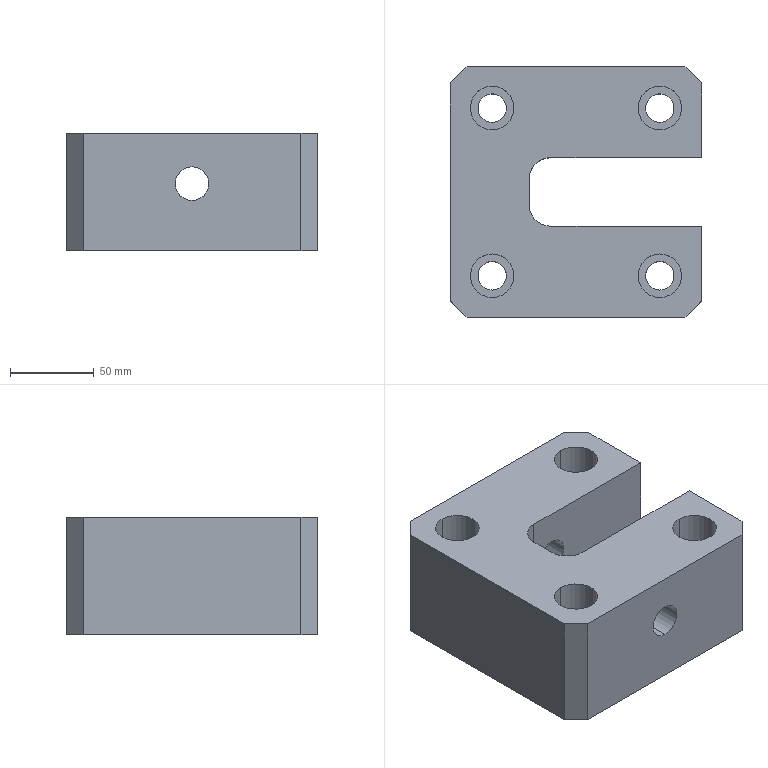Part | 1 solid | 40 faces | box 150 x 150 x 70 mm | volume 1149570 mm3 | cylinder 22 | plane 18 | commonest cylinder face diameters 26 x10 17 x8 20 x4